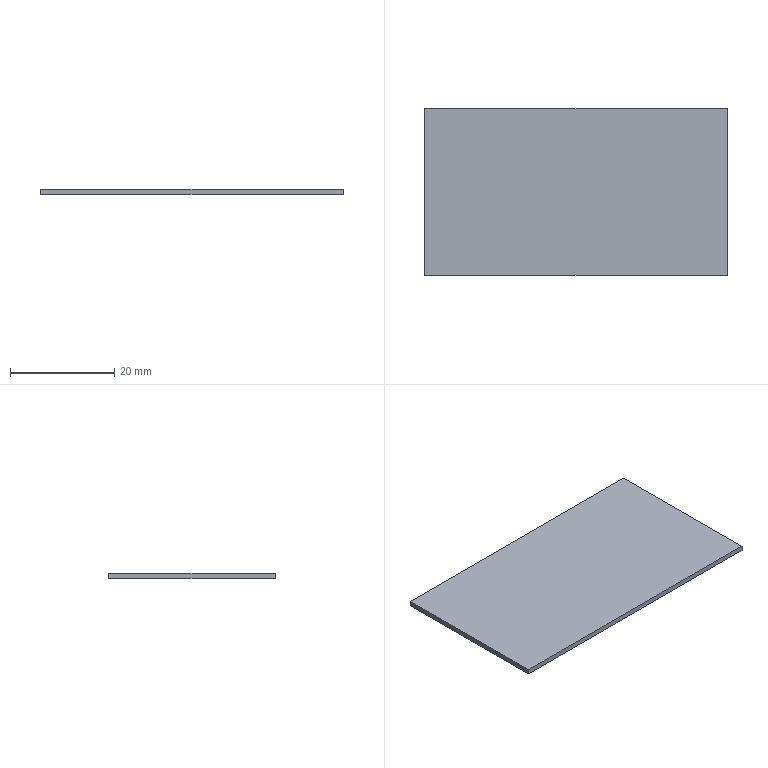Part | SolidWorks | features Extrusion 1 | 1 solid | 6 faces | box 58 x 32 x 1 mm | volume 1856 mm3 | plane 6
STEP:
#1=CARTESIAN_POINT('',(-29.,16.,0.5));
#2=VERTEX_POINT('',#1);
#3=CARTESIAN_POINT('',(-29.,-16.,0.5));
#4=VERTEX_POINT('',#3);
#5=CARTESIAN_POINT('',(-29.,16.,0.5));
#6=DIRECTION('',(0.,-1.,0.));
#7=VECTOR('',#6,1000.);
#8=LINE('',#5,#7);
#9=EDGE_CURVE('',#2,#4,#8,.T.);
#10=ORIENTED_EDGE('',*,*,#9,.F.);
#11=CARTESIAN_POINT('',(-29.,16.,-0.5));
#12=VERTEX_POINT('',#11);
#13=CARTESIAN_POINT('',(-29.,16.,-0.5));
#14=DIRECTION('',(0.,0.,1.));
#15=VECTOR('',#14,1000.);
#16=LINE('',#13,#15);
#17=EDGE_CURVE('',#12,#2,#16,.T.);
#18=ORIENTED_EDGE('',*,*,#17,.F.);
#19=CARTESIAN_POINT('',(-29.,-16.,-0.5));
#20=VERTEX_POINT('',#19);
#21=CARTESIAN_POINT('',(-29.,16.,-0.5));
#22=DIRECTION('',(0.,-1.,0.));
#23=VECTOR('',#22,1000.);
#24=LINE('',#21,#23);
#25=EDGE_CURVE('',#12,#20,#24,.T.);
#26=ORIENTED_EDGE('',*,*,#25,.T.);
#27=CARTESIAN_POINT('',(-29.,-16.,-0.5));
#28=DIRECTION('',(0.,0.,1.));
#29=VECTOR('',#28,1000.);
#30=LINE('',#27,#29);
#31=EDGE_CURVE('',#20,#4,#30,.T.);
#32=ORIENTED_EDGE('',*,*,#31,.T.);
#33=EDGE_LOOP('',(#10,#18,#26,#32));
#34=FACE_OUTER_BOUND('',#33,.T.);
#35=CARTESIAN_POINT('',(-29.,16.,-0.5));
#36=DIRECTION('',(-1.,0.,0.));
#37=DIRECTION('',(0.,0.,1.));
#38=AXIS2_PLACEMENT_3D('',#35,#36,#37);
#39=PLANE('',#38);
#40=ADVANCED_FACE('',(#34),#39,.T.);
#41=CARTESIAN_POINT('',(29.,16.,0.5));
#42=VERTEX_POINT('',#41);
#43=CARTESIAN_POINT('',(29.,16.,0.5));
#44=DIRECTION('',(-1.,0.,0.));
#45=VECTOR('',#44,1000.);
#46=LINE('',#43,#45);
#47=EDGE_CURVE('',#42,#2,#46,.T.);
#48=ORIENTED_EDGE('',*,*,#47,.F.);
#49=CARTESIAN_POINT('',(29.,16.,-0.5));
#50=VERTEX_POINT('',#49);
#51=CARTESIAN_POINT('',(29.,16.,-0.5));
#52=DIRECTION('',(0.,0.,1.));
#53=VECTOR('',#52,1000.);
#54=LINE('',#51,#53);
#55=EDGE_CURVE('',#50,#42,#54,.T.);
#56=ORIENTED_EDGE('',*,*,#55,.F.);
#57=CARTESIAN_POINT('',(29.,16.,-0.5));
#58=DIRECTION('',(-1.,0.,0.));
#59=VECTOR('',#58,1000.);
#60=LINE('',#57,#59);
#61=EDGE_CURVE('',#50,#12,#60,.T.);
#62=ORIENTED_EDGE('',*,*,#61,.T.);
#63=ORIENTED_EDGE('',*,*,#17,.T.);
#64=EDGE_LOOP('',(#48,#56,#62,#63));
#65=FACE_OUTER_BOUND('',#64,.T.);
#66=CARTESIAN_POINT('',(29.,16.,-0.5));
#67=DIRECTION('',(0.,1.,0.));
#68=DIRECTION('',(0.,0.,1.));
#69=AXIS2_PLACEMENT_3D('',#66,#67,#68);
#70=PLANE('',#69);
#71=ADVANCED_FACE('',(#65),#70,.T.);
#72=CARTESIAN_POINT('',(29.,-16.,0.5));
#73=VERTEX_POINT('',#72);
#74=CARTESIAN_POINT('',(29.,-16.,0.5));
#75=DIRECTION('',(0.,1.,0.));
#76=VECTOR('',#75,1000.);
#77=LINE('',#74,#76);
#78=EDGE_CURVE('',#73,#42,#77,.T.);
#79=ORIENTED_EDGE('',*,*,#78,.F.);
#80=CARTESIAN_POINT('',(29.,-16.,-0.5));
#81=VERTEX_POINT('',#80);
#82=CARTESIAN_POINT('',(29.,-16.,-0.5));
#83=DIRECTION('',(0.,0.,1.));
#84=VECTOR('',#83,1000.);
#85=LINE('',#82,#84);
#86=EDGE_CURVE('',#81,#73,#85,.T.);
#87=ORIENTED_EDGE('',*,*,#86,.F.);
#88=CARTESIAN_POINT('',(29.,-16.,-0.5));
#89=DIRECTION('',(0.,1.,0.));
#90=VECTOR('',#89,1000.);
#91=LINE('',#88,#90);
#92=EDGE_CURVE('',#81,#50,#91,.T.);
#93=ORIENTED_EDGE('',*,*,#92,.T.);
#94=ORIENTED_EDGE('',*,*,#55,.T.);
#95=EDGE_LOOP('',(#79,#87,#93,#94));
#96=FACE_OUTER_BOUND('',#95,.T.);
#97=CARTESIAN_POINT('',(29.,-16.,-0.5));
#98=DIRECTION('',(1.,0.,0.));
#99=DIRECTION('',(0.,0.,-1.));
#100=AXIS2_PLACEMENT_3D('',#97,#98,#99);
#101=PLANE('',#100);
#102=ADVANCED_FACE('',(#96),#101,.T.);
#103=CARTESIAN_POINT('',(-29.,-16.,0.5));
#104=DIRECTION('',(1.,0.,0.));
#105=VECTOR('',#104,1000.);
#106=LINE('',#103,#105);
#107=EDGE_CURVE('',#4,#73,#106,.T.);
#108=ORIENTED_EDGE('',*,*,#107,.F.);
#109=ORIENTED_EDGE('',*,*,#31,.F.);
#110=CARTESIAN_POINT('',(-29.,-16.,-0.5));
#111=DIRECTION('',(1.,0.,0.));
#112=VECTOR('',#111,1000.);
#113=LINE('',#110,#112);
#114=EDGE_CURVE('',#20,#81,#113,.T.);
#115=ORIENTED_EDGE('',*,*,#114,.T.);
#116=ORIENTED_EDGE('',*,*,#86,.T.);
#117=EDGE_LOOP('',(#108,#109,#115,#116));
#118=FACE_OUTER_BOUND('',#117,.T.);
#119=CARTESIAN_POINT('',(-29.,-16.,-0.5));
#120=DIRECTION('',(0.,-1.,0.));
#121=DIRECTION('',(0.,0.,-1.));
#122=AXIS2_PLACEMENT_3D('',#119,#120,#121);
#123=PLANE('',#122);
#124=ADVANCED_FACE('',(#118),#123,.T.);
#125=ORIENTED_EDGE('',*,*,#25,.F.);
#126=ORIENTED_EDGE('',*,*,#61,.F.);
#127=ORIENTED_EDGE('',*,*,#92,.F.);
#128=ORIENTED_EDGE('',*,*,#114,.F.);
#129=EDGE_LOOP('',(#125,#126,#127,#128));
#130=FACE_OUTER_BOUND('',#129,.T.);
#131=CARTESIAN_POINT('',(0.,0.,-0.5));
#132=DIRECTION('',(0.,0.,1.));
#133=DIRECTION('',(1.,0.,0.));
#134=AXIS2_PLACEMENT_3D('',#131,#132,#133);
#135=PLANE('',#134);
#136=ADVANCED_FACE('',(#130),#135,.F.);
#137=ORIENTED_EDGE('',*,*,#9,.T.);
#138=ORIENTED_EDGE('',*,*,#107,.T.);
#139=ORIENTED_EDGE('',*,*,#78,.T.);
#140=ORIENTED_EDGE('',*,*,#47,.T.);
#141=EDGE_LOOP('',(#137,#138,#139,#140));
#142=FACE_OUTER_BOUND('',#141,.T.);
#143=CARTESIAN_POINT('',(0.,0.,0.5));
#144=DIRECTION('',(0.,0.,1.));
#145=DIRECTION('',(1.,0.,0.));
#146=AXIS2_PLACEMENT_3D('',#143,#144,#145);
#147=PLANE('',#146);
#148=ADVANCED_FACE('',(#142),#147,.T.);
#149=CLOSED_SHELL('',(#40,#71,#102,#124,#136,#148));
#150=MANIFOLD_SOLID_BREP('',#149);
#151=CARTESIAN_POINT('',(0.,0.,0.));
#152=DIRECTION('',(0.,0.,1.));
#153=DIRECTION('',(1.,0.,0.));
#154=AXIS2_PLACEMENT_3D('',#151,#152,#153);
#155=(LENGTH_UNIT()NAMED_UNIT(*)SI_UNIT(.MILLI.,.METRE.));
#156=UNCERTAINTY_MEASURE_WITH_UNIT(LENGTH_MEASURE(0.00001),#155,'','');
#157=(NAMED_UNIT(*)PLANE_ANGLE_UNIT()SI_UNIT($,.RADIAN.));
#158=(NAMED_UNIT(*)SI_UNIT($,.STERADIAN.)SOLID_ANGLE_UNIT());
#159=(GEOMETRIC_REPRESENTATION_CONTEXT(3)GLOBAL_UNCERTAINTY_ASSIGNED_CONTEXT((#156))GLOBAL_UNIT_ASSIGNED_CONTEXT((#155,#157,#158))REPRESENTATION_CONTEXT('',''));
#160=ADVANCED_BREP_SHAPE_REPRESENTATION('',(#150,#154),#159);